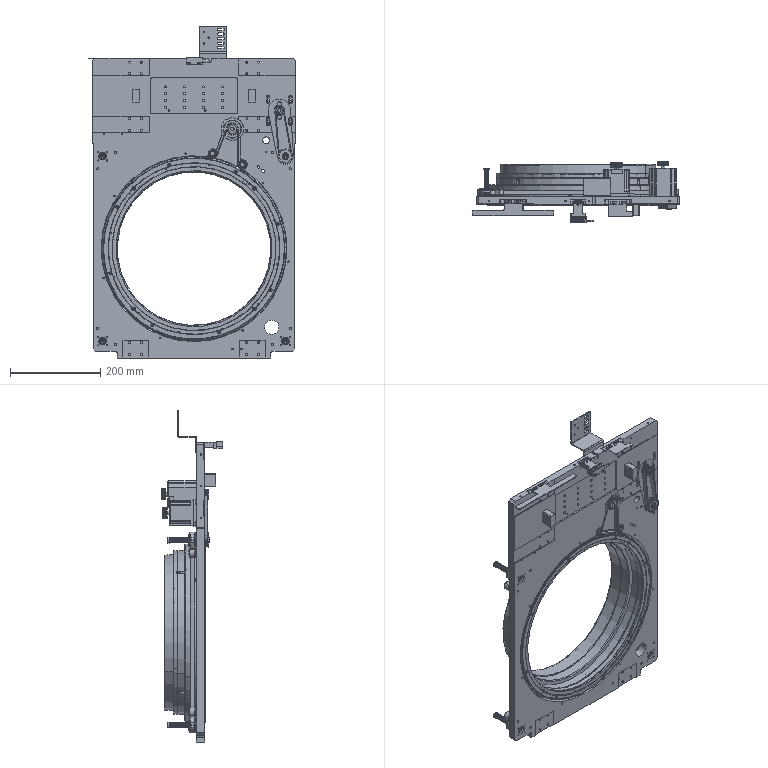Part | NX | features BREP 53 | 189 solids | 13811 faces | volume 4419914 mm3 | cylinder 7548 | plane 3788 | cone 1207 | sphere 592 | torus 572 | spline 104 | commonest cylinder face diameters 3.04 x1048 0.5 x1022 25 x742 1.7 x649 396.69 x416 1.02 x399